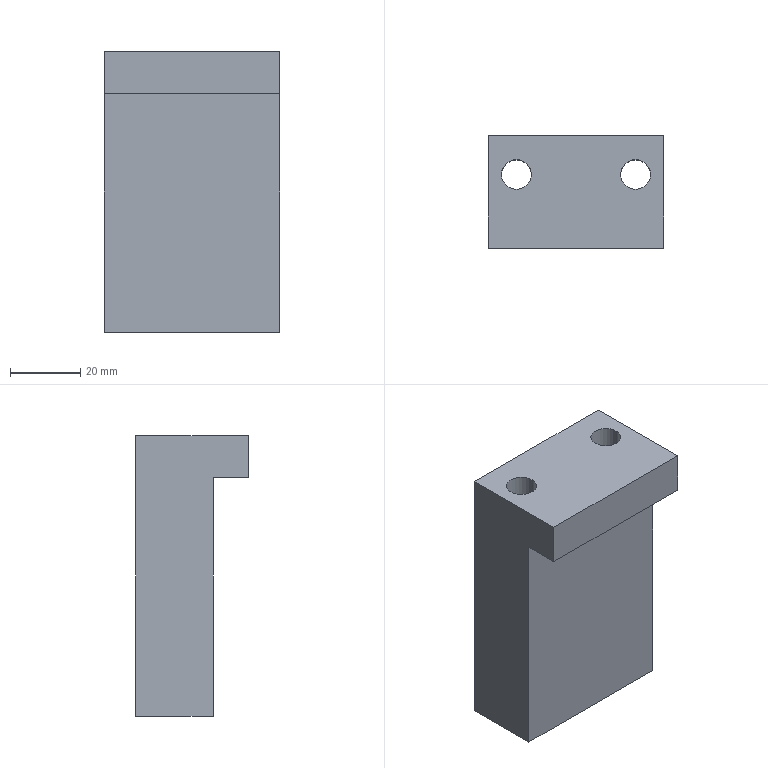Part | Creo | features DATUM PLANE 3, CURVE 2, PROTRUSION 2, COORDINATE SYSTEM 1 | 1 solid | 12 faces | box 50 x 32 x 80 mm | volume 84921 mm3 | plane 8 | cylinder 4 | commonest cylinder face diameters 8.5 x4
STEP:
#1=CARTESIAN_POINT('',(0.,0.,0.));
#2=DIRECTION('',(0.,0.,1.));
#3=DIRECTION('',(1.,0.,0.));
#4=AXIS2_PLACEMENT_3D('',#1,#2,#3);
#5=CARTESIAN_POINT('',(25.,-11.,0.));
#6=VERTEX_POINT('',#5);
#7=CARTESIAN_POINT('',(25.,11.,0.));
#8=VERTEX_POINT('',#7);
#9=CARTESIAN_POINT('',(25.,-11.,0.));
#10=DIRECTION('',(0.,1.,0.));
#11=VECTOR('',#10,22.);
#12=LINE('',#9,#11);
#13=EDGE_CURVE('',#6,#8,#12,.T.);
#14=ORIENTED_EDGE('',*,*,#13,.T.);
#15=CARTESIAN_POINT('',(-25.,11.,0.));
#16=VERTEX_POINT('',#15);
#17=CARTESIAN_POINT('',(25.,11.,0.));
#18=DIRECTION('',(-1.,0.,0.));
#19=VECTOR('',#18,50.);
#20=LINE('',#17,#19);
#21=EDGE_CURVE('',#8,#16,#20,.T.);
#22=ORIENTED_EDGE('',*,*,#21,.T.);
#23=CARTESIAN_POINT('',(-25.,-11.,0.));
#24=VERTEX_POINT('',#23);
#25=CARTESIAN_POINT('',(-25.,11.,0.));
#26=DIRECTION('',(0.,-1.,0.));
#27=VECTOR('',#26,22.);
#28=LINE('',#25,#27);
#29=EDGE_CURVE('',#16,#24,#28,.T.);
#30=ORIENTED_EDGE('',*,*,#29,.T.);
#31=CARTESIAN_POINT('',(-25.,-11.,0.));
#32=DIRECTION('',(1.,0.,0.));
#33=VECTOR('',#32,50.);
#34=LINE('',#31,#33);
#35=EDGE_CURVE('',#24,#6,#34,.T.);
#36=ORIENTED_EDGE('',*,*,#35,.T.);
#37=EDGE_LOOP('',(#14,#22,#30,#36));
#38=FACE_OUTER_BOUND('',#37,.F.);
#39=CARTESIAN_POINT('',(-12.75,0.,0.));
#40=VERTEX_POINT('',#39);
#41=CARTESIAN_POINT('',(-21.25,0.,0.));
#42=VERTEX_POINT('',#41);
#43=CARTESIAN_POINT('',(-17.,0.,0.));
#44=DIRECTION('',(0.,0.,-1.));
#45=DIRECTION('',(1.,0.,0.));
#46=AXIS2_PLACEMENT_3D('',#43,#44,#45);
#47=CIRCLE('',#46,4.25);
#48=EDGE_CURVE('',#40,#42,#47,.T.);
#49=ORIENTED_EDGE('',*,*,#48,.T.);
#50=CARTESIAN_POINT('',(-17.,0.,0.));
#51=DIRECTION('',(0.,0.,-1.));
#52=DIRECTION('',(-1.,0.,0.));
#53=AXIS2_PLACEMENT_3D('',#50,#51,#52);
#54=CIRCLE('',#53,4.25);
#55=EDGE_CURVE('',#42,#40,#54,.T.);
#56=ORIENTED_EDGE('',*,*,#55,.T.);
#57=EDGE_LOOP('',(#49,#56));
#58=FACE_BOUND('',#57,.F.);
#59=CARTESIAN_POINT('',(21.25,0.,0.));
#60=VERTEX_POINT('',#59);
#61=CARTESIAN_POINT('',(12.75,0.,0.));
#62=VERTEX_POINT('',#61);
#63=CARTESIAN_POINT('',(17.,0.,0.));
#64=DIRECTION('',(0.,0.,-1.));
#65=DIRECTION('',(1.,0.,0.));
#66=AXIS2_PLACEMENT_3D('',#63,#64,#65);
#67=CIRCLE('',#66,4.25);
#68=EDGE_CURVE('',#60,#62,#67,.T.);
#69=ORIENTED_EDGE('',*,*,#68,.T.);
#70=CARTESIAN_POINT('',(17.,0.,0.));
#71=DIRECTION('',(0.,0.,-1.));
#72=DIRECTION('',(-1.,0.,0.));
#73=AXIS2_PLACEMENT_3D('',#70,#71,#72);
#74=CIRCLE('',#73,4.25);
#75=EDGE_CURVE('',#62,#60,#74,.T.);
#76=ORIENTED_EDGE('',*,*,#75,.T.);
#77=EDGE_LOOP('',(#69,#76));
#78=FACE_BOUND('',#77,.F.);
#79=CARTESIAN_POINT('',(0.,0.,0.));
#80=DIRECTION('',(0.,0.,1.));
#81=DIRECTION('',(1.,0.,0.));
#82=AXIS2_PLACEMENT_3D('',#79,#80,#81);
#83=PLANE('',#82);
#84=ADVANCED_FACE('',(#38,#58,#78),#83,.F.);
#85=ORIENTED_EDGE('',*,*,#68,.F.);
#86=CARTESIAN_POINT('',(21.25,0.,80.));
#87=VERTEX_POINT('',#86);
#88=CARTESIAN_POINT('',(21.25,0.,0.));
#89=DIRECTION('',(0.,0.,1.));
#90=VECTOR('',#89,80.);
#91=LINE('',#88,#90);
#92=EDGE_CURVE('',#60,#87,#91,.T.);
#93=ORIENTED_EDGE('',*,*,#92,.T.);
#94=CARTESIAN_POINT('',(12.75,0.,80.));
#95=VERTEX_POINT('',#94);
#96=CARTESIAN_POINT('',(17.,0.,80.));
#97=DIRECTION('',(0.,0.,-1.));
#98=DIRECTION('',(1.,0.,0.));
#99=AXIS2_PLACEMENT_3D('',#96,#97,#98);
#100=CIRCLE('',#99,4.25);
#101=EDGE_CURVE('',#87,#95,#100,.T.);
#102=ORIENTED_EDGE('',*,*,#101,.T.);
#103=CARTESIAN_POINT('',(12.75,0.,0.));
#104=DIRECTION('',(0.,0.,1.));
#105=VECTOR('',#104,80.);
#106=LINE('',#103,#105);
#107=EDGE_CURVE('',#62,#95,#106,.T.);
#108=ORIENTED_EDGE('',*,*,#107,.F.);
#109=EDGE_LOOP('',(#85,#93,#102,#108));
#110=FACE_OUTER_BOUND('',#109,.F.);
#111=CARTESIAN_POINT('',(17.,0.,0.));
#112=DIRECTION('',(0.,0.,1.));
#113=DIRECTION('',(1.,0.,0.));
#114=AXIS2_PLACEMENT_3D('',#111,#112,#113);
#115=CYLINDRICAL_SURFACE('',#114,4.25);
#116=ADVANCED_FACE('',(#110),#115,.F.);
#117=ORIENTED_EDGE('',*,*,#75,.F.);
#118=ORIENTED_EDGE('',*,*,#107,.T.);
#119=CARTESIAN_POINT('',(17.,0.,80.));
#120=DIRECTION('',(0.,0.,-1.));
#121=DIRECTION('',(-1.,0.,0.));
#122=AXIS2_PLACEMENT_3D('',#119,#120,#121);
#123=CIRCLE('',#122,4.25);
#124=EDGE_CURVE('',#95,#87,#123,.T.);
#125=ORIENTED_EDGE('',*,*,#124,.T.);
#126=ORIENTED_EDGE('',*,*,#92,.F.);
#127=EDGE_LOOP('',(#117,#118,#125,#126));
#128=FACE_OUTER_BOUND('',#127,.F.);
#129=CARTESIAN_POINT('',(17.,0.,0.));
#130=DIRECTION('',(0.,0.,1.));
#131=DIRECTION('',(1.,0.,0.));
#132=AXIS2_PLACEMENT_3D('',#129,#130,#131);
#133=CYLINDRICAL_SURFACE('',#132,4.25);
#134=ADVANCED_FACE('',(#128),#133,.F.);
#135=CARTESIAN_POINT('',(25.,11.,80.));
#136=VERTEX_POINT('',#135);
#137=CARTESIAN_POINT('',(25.,-21.,80.));
#138=VERTEX_POINT('',#137);
#139=CARTESIAN_POINT('',(25.,11.,80.));
#140=DIRECTION('',(0.,-1.,0.));
#141=VECTOR('',#140,32.);
#142=LINE('',#139,#141);
#143=EDGE_CURVE('',#136,#138,#142,.T.);
#144=ORIENTED_EDGE('',*,*,#143,.T.);
#145=CARTESIAN_POINT('',(-25.,-21.,80.));
#146=VERTEX_POINT('',#145);
#147=CARTESIAN_POINT('',(25.,-21.,80.));
#148=DIRECTION('',(-1.,0.,0.));
#149=VECTOR('',#148,50.);
#150=LINE('',#147,#149);
#151=EDGE_CURVE('',#138,#146,#150,.T.);
#152=ORIENTED_EDGE('',*,*,#151,.T.);
#153=CARTESIAN_POINT('',(-25.,11.,80.));
#154=VERTEX_POINT('',#153);
#155=CARTESIAN_POINT('',(-25.,11.,80.));
#156=DIRECTION('',(0.,-1.,0.));
#157=VECTOR('',#156,32.);
#158=LINE('',#155,#157);
#159=EDGE_CURVE('',#154,#146,#158,.T.);
#160=ORIENTED_EDGE('',*,*,#159,.F.);
#161=CARTESIAN_POINT('',(25.,11.,80.));
#162=DIRECTION('',(-1.,0.,0.));
#163=VECTOR('',#162,50.);
#164=LINE('',#161,#163);
#165=EDGE_CURVE('',#136,#154,#164,.T.);
#166=ORIENTED_EDGE('',*,*,#165,.F.);
#167=EDGE_LOOP('',(#144,#152,#160,#166));
#168=FACE_OUTER_BOUND('',#167,.F.);
#169=CARTESIAN_POINT('',(-12.75,0.,80.));
#170=VERTEX_POINT('',#169);
#171=CARTESIAN_POINT('',(-21.25,0.,80.));
#172=VERTEX_POINT('',#171);
#173=CARTESIAN_POINT('',(-17.,0.,80.));
#174=DIRECTION('',(0.,0.,-1.));
#175=DIRECTION('',(1.,0.,0.));
#176=AXIS2_PLACEMENT_3D('',#173,#174,#175);
#177=CIRCLE('',#176,4.25);
#178=EDGE_CURVE('',#170,#172,#177,.T.);
#179=ORIENTED_EDGE('',*,*,#178,.F.);
#180=CARTESIAN_POINT('',(-17.,0.,80.));
#181=DIRECTION('',(0.,0.,-1.));
#182=DIRECTION('',(-1.,0.,0.));
#183=AXIS2_PLACEMENT_3D('',#180,#181,#182);
#184=CIRCLE('',#183,4.25);
#185=EDGE_CURVE('',#172,#170,#184,.T.);
#186=ORIENTED_EDGE('',*,*,#185,.F.);
#187=EDGE_LOOP('',(#179,#186));
#188=FACE_BOUND('',#187,.F.);
#189=ORIENTED_EDGE('',*,*,#101,.F.);
#190=ORIENTED_EDGE('',*,*,#124,.F.);
#191=EDGE_LOOP('',(#189,#190));
#192=FACE_BOUND('',#191,.F.);
#193=CARTESIAN_POINT('',(0.,0.,80.));
#194=DIRECTION('',(0.,0.,1.));
#195=DIRECTION('',(1.,0.,0.));
#196=AXIS2_PLACEMENT_3D('',#193,#194,#195);
#197=PLANE('',#196);
#198=ADVANCED_FACE('',(#168,#188,#192),#197,.T.);
#199=ORIENTED_EDGE('',*,*,#48,.F.);
#200=CARTESIAN_POINT('',(-12.75,0.,0.));
#201=DIRECTION('',(0.,0.,1.));
#202=VECTOR('',#201,80.);
#203=LINE('',#200,#202);
#204=EDGE_CURVE('',#40,#170,#203,.T.);
#205=ORIENTED_EDGE('',*,*,#204,.T.);
#206=ORIENTED_EDGE('',*,*,#178,.T.);
#207=CARTESIAN_POINT('',(-21.25,0.,0.));
#208=DIRECTION('',(0.,0.,1.));
#209=VECTOR('',#208,80.);
#210=LINE('',#207,#209);
#211=EDGE_CURVE('',#42,#172,#210,.T.);
#212=ORIENTED_EDGE('',*,*,#211,.F.);
#213=EDGE_LOOP('',(#199,#205,#206,#212));
#214=FACE_OUTER_BOUND('',#213,.F.);
#215=CARTESIAN_POINT('',(-17.,0.,0.));
#216=DIRECTION('',(0.,0.,1.));
#217=DIRECTION('',(1.,0.,0.));
#218=AXIS2_PLACEMENT_3D('',#215,#216,#217);
#219=CYLINDRICAL_SURFACE('',#218,4.25);
#220=ADVANCED_FACE('',(#214),#219,.F.);
#221=ORIENTED_EDGE('',*,*,#55,.F.);
#222=ORIENTED_EDGE('',*,*,#211,.T.);
#223=ORIENTED_EDGE('',*,*,#185,.T.);
#224=ORIENTED_EDGE('',*,*,#204,.F.);
#225=EDGE_LOOP('',(#221,#222,#223,#224));
#226=FACE_OUTER_BOUND('',#225,.F.);
#227=CARTESIAN_POINT('',(-17.,0.,0.));
#228=DIRECTION('',(0.,0.,1.));
#229=DIRECTION('',(1.,0.,0.));
#230=AXIS2_PLACEMENT_3D('',#227,#228,#229);
#231=CYLINDRICAL_SURFACE('',#230,4.25);
#232=ADVANCED_FACE('',(#226),#231,.F.);
#233=CARTESIAN_POINT('',(25.,-11.,68.));
#234=VERTEX_POINT('',#233);
#235=CARTESIAN_POINT('',(25.,-11.,0.));
#236=DIRECTION('',(0.,0.,1.));
#237=VECTOR('',#236,68.);
#238=LINE('',#235,#237);
#239=EDGE_CURVE('',#6,#234,#238,.T.);
#240=ORIENTED_EDGE('',*,*,#239,.T.);
#241=CARTESIAN_POINT('',(25.,-21.,68.));
#242=VERTEX_POINT('',#241);
#243=CARTESIAN_POINT('',(25.,-11.,68.));
#244=DIRECTION('',(0.,-1.,0.));
#245=VECTOR('',#244,10.);
#246=LINE('',#243,#245);
#247=EDGE_CURVE('',#234,#242,#246,.T.);
#248=ORIENTED_EDGE('',*,*,#247,.T.);
#249=CARTESIAN_POINT('',(25.,-21.,68.));
#250=DIRECTION('',(0.,0.,1.));
#251=VECTOR('',#250,12.);
#252=LINE('',#249,#251);
#253=EDGE_CURVE('',#242,#138,#252,.T.);
#254=ORIENTED_EDGE('',*,*,#253,.T.);
#255=ORIENTED_EDGE('',*,*,#143,.F.);
#256=CARTESIAN_POINT('',(25.,11.,0.));
#257=DIRECTION('',(0.,0.,1.));
#258=VECTOR('',#257,80.);
#259=LINE('',#256,#258);
#260=EDGE_CURVE('',#8,#136,#259,.T.);
#261=ORIENTED_EDGE('',*,*,#260,.F.);
#262=ORIENTED_EDGE('',*,*,#13,.F.);
#263=EDGE_LOOP('',(#240,#248,#254,#255,#261,#262));
#264=FACE_OUTER_BOUND('',#263,.F.);
#265=CARTESIAN_POINT('',(25.,-11.,0.));
#266=DIRECTION('',(1.,0.,0.));
#267=DIRECTION('',(0.,1.,0.));
#268=AXIS2_PLACEMENT_3D('',#265,#266,#267);
#269=PLANE('',#268);
#270=ADVANCED_FACE('',(#264),#269,.T.);
#271=CARTESIAN_POINT('',(-25.,-11.,68.));
#272=VERTEX_POINT('',#271);
#273=CARTESIAN_POINT('',(-25.,-11.,68.));
#274=DIRECTION('',(1.,0.,0.));
#275=VECTOR('',#274,50.);
#276=LINE('',#273,#275);
#277=EDGE_CURVE('',#272,#234,#276,.T.);
#278=ORIENTED_EDGE('',*,*,#277,.T.);
#279=ORIENTED_EDGE('',*,*,#239,.F.);
#280=ORIENTED_EDGE('',*,*,#35,.F.);
#281=CARTESIAN_POINT('',(-25.,-11.,0.));
#282=DIRECTION('',(0.,0.,1.));
#283=VECTOR('',#282,68.);
#284=LINE('',#281,#283);
#285=EDGE_CURVE('',#24,#272,#284,.T.);
#286=ORIENTED_EDGE('',*,*,#285,.T.);
#287=EDGE_LOOP('',(#278,#279,#280,#286));
#288=FACE_OUTER_BOUND('',#287,.F.);
#289=CARTESIAN_POINT('',(-25.,-11.,0.));
#290=DIRECTION('',(0.,-1.,0.));
#291=DIRECTION('',(1.,0.,0.));
#292=AXIS2_PLACEMENT_3D('',#289,#290,#291);
#293=PLANE('',#292);
#294=ADVANCED_FACE('',(#288),#293,.T.);
#295=ORIENTED_EDGE('',*,*,#277,.F.);
#296=CARTESIAN_POINT('',(-25.,-21.,68.));
#297=VERTEX_POINT('',#296);
#298=CARTESIAN_POINT('',(-25.,-11.,68.));
#299=DIRECTION('',(0.,-1.,0.));
#300=VECTOR('',#299,10.);
#301=LINE('',#298,#300);
#302=EDGE_CURVE('',#272,#297,#301,.T.);
#303=ORIENTED_EDGE('',*,*,#302,.T.);
#304=CARTESIAN_POINT('',(-25.,-21.,68.));
#305=DIRECTION('',(1.,0.,0.));
#306=VECTOR('',#305,50.);
#307=LINE('',#304,#306);
#308=EDGE_CURVE('',#297,#242,#307,.T.);
#309=ORIENTED_EDGE('',*,*,#308,.T.);
#310=ORIENTED_EDGE('',*,*,#247,.F.);
#311=EDGE_LOOP('',(#295,#303,#309,#310));
#312=FACE_OUTER_BOUND('',#311,.F.);
#313=CARTESIAN_POINT('',(-25.,-11.,68.));
#314=DIRECTION('',(0.,0.,-1.));
#315=DIRECTION('',(1.,0.,0.));
#316=AXIS2_PLACEMENT_3D('',#313,#314,#315);
#317=PLANE('',#316);
#318=ADVANCED_FACE('',(#312),#317,.T.);
#319=ORIENTED_EDGE('',*,*,#159,.T.);
#320=CARTESIAN_POINT('',(-25.,-21.,80.));
#321=DIRECTION('',(0.,0.,-1.));
#322=VECTOR('',#321,12.);
#323=LINE('',#320,#322);
#324=EDGE_CURVE('',#146,#297,#323,.T.);
#325=ORIENTED_EDGE('',*,*,#324,.T.);
#326=ORIENTED_EDGE('',*,*,#302,.F.);
#327=ORIENTED_EDGE('',*,*,#285,.F.);
#328=ORIENTED_EDGE('',*,*,#29,.F.);
#329=CARTESIAN_POINT('',(-25.,11.,0.));
#330=DIRECTION('',(0.,0.,1.));
#331=VECTOR('',#330,80.);
#332=LINE('',#329,#331);
#333=EDGE_CURVE('',#16,#154,#332,.T.);
#334=ORIENTED_EDGE('',*,*,#333,.T.);
#335=EDGE_LOOP('',(#319,#325,#326,#327,#328,#334));
#336=FACE_OUTER_BOUND('',#335,.F.);
#337=CARTESIAN_POINT('',(-25.,11.,0.));
#338=DIRECTION('',(-1.,0.,0.));
#339=DIRECTION('',(0.,-1.,0.));
#340=AXIS2_PLACEMENT_3D('',#337,#338,#339);
#341=PLANE('',#340);
#342=ADVANCED_FACE('',(#336),#341,.T.);
#343=ORIENTED_EDGE('',*,*,#308,.F.);
#344=ORIENTED_EDGE('',*,*,#324,.F.);
#345=ORIENTED_EDGE('',*,*,#151,.F.);
#346=ORIENTED_EDGE('',*,*,#253,.F.);
#347=EDGE_LOOP('',(#343,#344,#345,#346));
#348=FACE_OUTER_BOUND('',#347,.F.);
#349=CARTESIAN_POINT('',(0.,-21.,0.));
#350=DIRECTION('',(0.,-1.,0.));
#351=DIRECTION('',(1.,0.,0.));
#352=AXIS2_PLACEMENT_3D('',#349,#350,#351);
#353=PLANE('',#352);
#354=ADVANCED_FACE('',(#348),#353,.T.);
#355=ORIENTED_EDGE('',*,*,#21,.F.);
#356=ORIENTED_EDGE('',*,*,#260,.T.);
#357=ORIENTED_EDGE('',*,*,#165,.T.);
#358=ORIENTED_EDGE('',*,*,#333,.F.);
#359=EDGE_LOOP('',(#355,#356,#357,#358));
#360=FACE_OUTER_BOUND('',#359,.F.);
#361=CARTESIAN_POINT('',(25.,11.,0.));
#362=DIRECTION('',(0.,1.,0.));
#363=DIRECTION('',(-1.,0.,0.));
#364=AXIS2_PLACEMENT_3D('',#361,#362,#363);
#365=PLANE('',#364);
#366=ADVANCED_FACE('',(#360),#365,.T.);
#367=CLOSED_SHELL('',(#84,#116,#134,#198,#220,#232,#270,#294,#318,#342,#354,#366));
#368=MANIFOLD_SOLID_BREP('',#367);
#369=(LENGTH_UNIT()NAMED_UNIT(*)SI_UNIT(.MILLI.,.METRE.));
#370=UNCERTAINTY_MEASURE_WITH_UNIT(LENGTH_MEASURE(0.009962),#369,'','');
#371=(NAMED_UNIT(*)PLANE_ANGLE_UNIT()SI_UNIT($,.RADIAN.));
#372=PLANE_ANGLE_MEASURE_WITH_UNIT(PLANE_ANGLE_MEASURE(0.01745),#371);
#373=(CONVERSION_BASED_UNIT('DEGREE',#372)NAMED_UNIT(*)PLANE_ANGLE_UNIT());
#374=(NAMED_UNIT(*)SI_UNIT($,.STERADIAN.)SOLID_ANGLE_UNIT());
#375=(GEOMETRIC_REPRESENTATION_CONTEXT(3)GLOBAL_UNCERTAINTY_ASSIGNED_CONTEXT((#370))GLOBAL_UNIT_ASSIGNED_CONTEXT((#369,#373,#374))REPRESENTATION_CONTEXT('',''));
#376=ADVANCED_BREP_SHAPE_REPRESENTATION('',(#4,#368),#375);